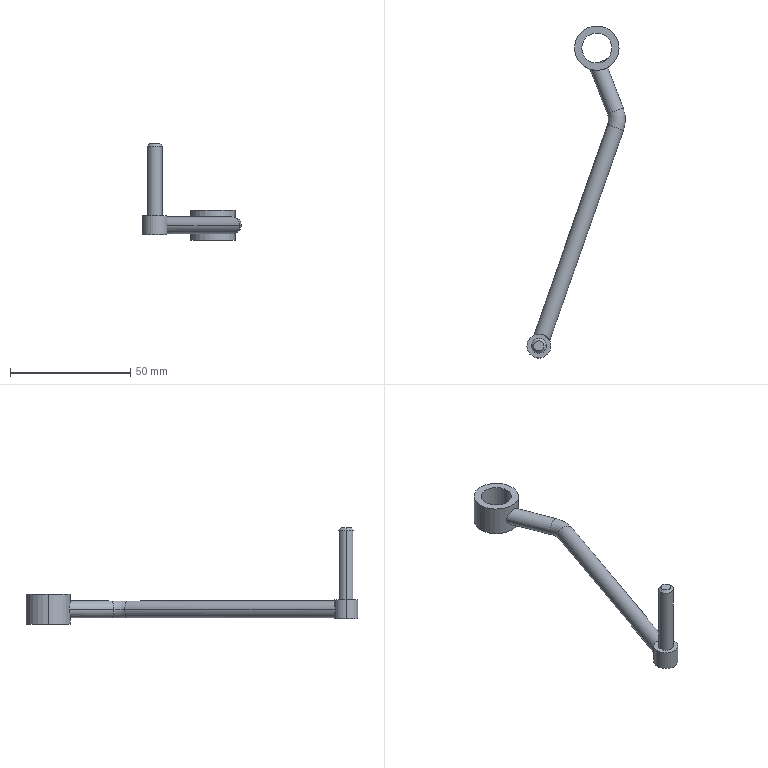Part | SolidWorks | features 3DProfileFeature 2, ICE 2, Chamfer 1, Extrusion 1, Sweep 1 | 1 solid | 24 faces | box 40.944 x 138.187 x 40.25 mm | volume 7860 mm3 | cylinder 14 | plane 6 | torus 2 | cone 2 | commonest cylinder face diameters 7 x6 6.192 x2 10 x2 12.5 x2 18.5 x2
STEP:
#1=CARTESIAN_POINT('',(4.41,-27.398,6.25));
#2=VERTEX_POINT('',#1);
#3=CARTESIAN_POINT('',(10.941,-24.878,6.25));
#4=VERTEX_POINT('',#3);
#5=CARTESIAN_POINT('',(7.675,-26.138,6.25));
#6=DIRECTION('',(0.3601,-0.9329,0.));
#7=DIRECTION('',(0.9329,0.3601,0.));
#8=AXIS2_PLACEMENT_3D('',#5,#6,#7);
#9=CIRCLE('',#8,3.5);
#10=EDGE_CURVE('',#2,#4,#9,.T.);
#11=ORIENTED_EDGE('',*,*,#10,.T.);
#12=CARTESIAN_POINT('',(11.085,-34.207,6.25));
#13=VERTEX_POINT('',#12);
#14=CARTESIAN_POINT('',(-1.654,-29.738,6.25));
#15=DIRECTION('',(0.,0.,-1.));
#16=DIRECTION('',(0.,1.,0.));
#17=AXIS2_PLACEMENT_3D('',#14,#15,#16);
#18=CIRCLE('',#17,13.5);
#19=EDGE_CURVE('',#4,#13,#18,.T.);
#20=ORIENTED_EDGE('',*,*,#19,.T.);
#21=CARTESIAN_POINT('',(4.48,-31.89,6.25));
#22=VERTEX_POINT('',#21);
#23=CARTESIAN_POINT('',(7.782,-33.048,6.25));
#24=DIRECTION('',(-0.331,-0.9436,0.));
#25=DIRECTION('',(0.9436,-0.331,0.));
#26=AXIS2_PLACEMENT_3D('',#23,#24,#25);
#27=CIRCLE('',#26,3.5);
#28=EDGE_CURVE('',#22,#13,#27,.T.);
#29=ORIENTED_EDGE('',*,*,#28,.F.);
#30=CARTESIAN_POINT('',(-1.654,-29.738,6.25));
#31=DIRECTION('',(0.,0.,-1.));
#32=DIRECTION('',(0.,1.,0.));
#33=AXIS2_PLACEMENT_3D('',#30,#31,#32);
#34=CIRCLE('',#33,6.5);
#35=EDGE_CURVE('',#2,#22,#34,.T.);
#36=ORIENTED_EDGE('',*,*,#35,.F.);
#37=EDGE_LOOP('',(#11,#20,#29,#36));
#38=FACE_OUTER_BOUND('',#37,.T.);
#39=CARTESIAN_POINT('',(-1.654,-29.738,6.25));
#40=DIRECTION('',(0.,0.,-1.));
#41=DIRECTION('',(0.,1.,0.));
#42=AXIS2_PLACEMENT_3D('',#39,#40,#41);
#43=TOROIDAL_SURFACE('',#42,10.,3.5);
#44=ADVANCED_FACE('',(#38),#43,.T.);
#45=CARTESIAN_POINT('',(-22.001,-123.937,40.25));
#46=VERTEX_POINT('',#45);
#47=CARTESIAN_POINT('',(-26.194,-123.937,40.25));
#48=VERTEX_POINT('',#47);
#49=CARTESIAN_POINT('',(-24.097,-123.937,40.25));
#50=DIRECTION('',(0.,0.,1.));
#51=DIRECTION('',(1.,0.,0.));
#52=AXIS2_PLACEMENT_3D('',#49,#50,#51);
#53=CIRCLE('',#52,2.096);
#54=EDGE_CURVE('',#46,#48,#53,.T.);
#55=ORIENTED_EDGE('',*,*,#54,.F.);
#56=CARTESIAN_POINT('',(-21.001,-123.937,39.25));
#57=VERTEX_POINT('',#56);
#58=CARTESIAN_POINT('',(-22.001,-123.937,40.25));
#59=DIRECTION('',(0.7071,0.,-0.7071));
#60=VECTOR('',#59,1000.);
#61=LINE('',#58,#60);
#62=EDGE_CURVE('',#46,#57,#61,.T.);
#63=ORIENTED_EDGE('',*,*,#62,.T.);
#64=CARTESIAN_POINT('',(-27.194,-123.937,39.25));
#65=VERTEX_POINT('',#64);
#66=CARTESIAN_POINT('',(-24.097,-123.937,39.25));
#67=DIRECTION('',(0.,0.,-1.));
#68=DIRECTION('',(1.,0.,0.));
#69=AXIS2_PLACEMENT_3D('',#66,#67,#68);
#70=CIRCLE('',#69,3.096);
#71=EDGE_CURVE('',#65,#57,#70,.T.);
#72=ORIENTED_EDGE('',*,*,#71,.F.);
#73=CARTESIAN_POINT('',(-26.194,-123.937,40.25));
#74=DIRECTION('',(-0.7071,0.,-0.7071));
#75=VECTOR('',#74,1000.);
#76=LINE('',#73,#75);
#77=EDGE_CURVE('',#48,#65,#76,.T.);
#78=ORIENTED_EDGE('',*,*,#77,.F.);
#79=EDGE_LOOP('',(#55,#63,#72,#78));
#80=FACE_OUTER_BOUND('',#79,.T.);
#81=CARTESIAN_POINT('',(-24.097,-123.937,40.25));
#82=DIRECTION('',(0.,0.,-1.));
#83=DIRECTION('',(-1.,0.,0.));
#84=AXIS2_PLACEMENT_3D('',#81,#82,#83);
#85=CONICAL_SURFACE('',#84,2.096,0.7854);
#86=ADVANCED_FACE('',(#80),#85,.T.);
#87=ORIENTED_EDGE('',*,*,#71,.T.);
#88=CARTESIAN_POINT('',(-21.001,-123.937,10.25));
#89=VERTEX_POINT('',#88);
#90=CARTESIAN_POINT('',(-21.001,-123.937,40.25));
#91=DIRECTION('',(0.,0.,-1.));
#92=VECTOR('',#91,1000.);
#93=LINE('',#90,#92);
#94=EDGE_CURVE('',#57,#89,#93,.T.);
#95=ORIENTED_EDGE('',*,*,#94,.T.);
#96=CARTESIAN_POINT('',(-27.194,-123.937,10.25));
#97=VERTEX_POINT('',#96);
#98=CARTESIAN_POINT('',(-24.097,-123.937,10.25));
#99=DIRECTION('',(0.,0.,1.));
#100=DIRECTION('',(1.,0.,0.));
#101=AXIS2_PLACEMENT_3D('',#98,#99,#100);
#102=CIRCLE('',#101,3.096);
#103=EDGE_CURVE('',#89,#97,#102,.T.);
#104=ORIENTED_EDGE('',*,*,#103,.T.);
#105=CARTESIAN_POINT('',(-27.194,-123.937,40.25));
#106=DIRECTION('',(0.,0.,-1.));
#107=VECTOR('',#106,1000.);
#108=LINE('',#105,#107);
#109=EDGE_CURVE('',#65,#97,#108,.T.);
#110=ORIENTED_EDGE('',*,*,#109,.F.);
#111=EDGE_LOOP('',(#87,#95,#104,#110));
#112=FACE_OUTER_BOUND('',#111,.T.);
#113=CARTESIAN_POINT('',(-24.097,-123.937,40.25));
#114=DIRECTION('',(0.,0.,-1.));
#115=DIRECTION('',(-1.,0.,0.));
#116=AXIS2_PLACEMENT_3D('',#113,#114,#115);
#117=CYLINDRICAL_SURFACE('',#116,3.096);
#118=ADVANCED_FACE('',(#112),#117,.T.);
#119=CARTESIAN_POINT('',(-19.613,-121.726,6.25));
#120=VERTEX_POINT('',#119);
#121=CARTESIAN_POINT('',(-26.218,-119.409,6.25));
#122=VERTEX_POINT('',#121);
#123=CARTESIAN_POINT('',(-19.613,-121.726,6.25));
#124=CARTESIAN_POINT('',(-19.613,-121.726,6.009));
#125=CARTESIAN_POINT('',(-19.628,-121.695,5.775));
#126=CARTESIAN_POINT('',(-19.687,-121.58,5.318));
#127=CARTESIAN_POINT('',(-19.732,-121.496,5.095));
#128=CARTESIAN_POINT('',(-19.849,-121.298,4.679));
#129=CARTESIAN_POINT('',(-19.922,-121.182,4.481));
#130=CARTESIAN_POINT('',(-20.097,-120.933,4.113));
#131=CARTESIAN_POINT('',(-20.199,-120.801,3.943));
#132=CARTESIAN_POINT('',(-20.433,-120.53,3.629));
#133=CARTESIAN_POINT('',(-20.567,-120.39,3.485));
#134=CARTESIAN_POINT('',(-20.862,-120.119,3.234));
#135=CARTESIAN_POINT('',(-21.024,-119.987,3.125));
#136=CARTESIAN_POINT('',(-21.382,-119.732,2.943));
#137=CARTESIAN_POINT('',(-21.58,-119.611,2.871));
#138=CARTESIAN_POINT('',(-21.992,-119.396,2.776));
#139=CARTESIAN_POINT('',(-22.213,-119.299,2.75));
#140=CARTESIAN_POINT('',(-22.664,-119.141,2.75));
#141=CARTESIAN_POINT('',(-22.891,-119.079,2.774));
#142=CARTESIAN_POINT('',(-23.351,-118.987,2.869));
#143=CARTESIAN_POINT('',(-23.58,-118.959,2.94));
#144=CARTESIAN_POINT('',(-24.02,-118.933,3.12));
#145=CARTESIAN_POINT('',(-24.235,-118.935,3.231));
#146=CARTESIAN_POINT('',(-24.638,-118.962,3.484));
#147=CARTESIAN_POINT('',(-24.828,-118.987,3.626));
#148=CARTESIAN_POINT('',(-25.183,-119.053,3.942));
#149=CARTESIAN_POINT('',(-25.345,-119.093,4.113));
#150=CARTESIAN_POINT('',(-25.635,-119.177,4.479));
#151=CARTESIAN_POINT('',(-25.765,-119.222,4.676));
#152=CARTESIAN_POINT('',(-25.982,-119.304,5.095));
#153=CARTESIAN_POINT('',(-26.068,-119.341,5.314));
#154=CARTESIAN_POINT('',(-26.157,-119.381,5.659));
#155=CARTESIAN_POINT('',(-26.18,-119.391,5.777));
#156=CARTESIAN_POINT('',(-26.211,-119.405,6.013));
#157=CARTESIAN_POINT('',(-26.218,-119.409,6.132));
#158=CARTESIAN_POINT('',(-26.218,-119.409,6.25));
#159=B_SPLINE_CURVE_WITH_KNOTS('',3,(#123,#124,#125,#126,#127,#128,#129,#130,#131,#132,#133,#134,#135,#136,#137,#138,#139,#140,#141,#142,#143,#144,#145,#146,#147,#148,#149,#150,#151,#152,#153,#154,#155,#156,#157,#158),.UNSPECIFIED.,.F.,.F.,(4,2,2,2,2,2,2,2,2,2,2,2,2,2,2,2,2,4),(0.,0.0007095,0.001419,0.002128,0.002838,0.003547,0.004257,0.004966,0.005676,0.006385,0.007095,0.007804,0.008514,0.009223,0.009933,0.01064,0.011,0.01135),.UNSPECIFIED.);
#160=EDGE_CURVE('',#120,#122,#159,.T.);
#161=ORIENTED_EDGE('',*,*,#160,.F.);
#162=CARTESIAN_POINT('',(-26.218,-119.409,6.25));
#163=CARTESIAN_POINT('',(-26.218,-119.409,6.486));
#164=CARTESIAN_POINT('',(-26.187,-119.394,6.727));
#165=CARTESIAN_POINT('',(-26.068,-119.341,7.186));
#166=CARTESIAN_POINT('',(-25.981,-119.304,7.407));
#167=CARTESIAN_POINT('',(-25.764,-119.221,7.826));
#168=CARTESIAN_POINT('',(-25.636,-119.177,8.02));
#169=CARTESIAN_POINT('',(-25.346,-119.093,8.386));
#170=CARTESIAN_POINT('',(-25.182,-119.053,8.559));
#171=CARTESIAN_POINT('',(-24.83,-118.987,8.872));
#172=CARTESIAN_POINT('',(-24.641,-118.962,9.013));
#173=CARTESIAN_POINT('',(-24.239,-118.935,9.266));
#174=CARTESIAN_POINT('',(-24.024,-118.933,9.378));
#175=CARTESIAN_POINT('',(-23.586,-118.958,9.558));
#176=CARTESIAN_POINT('',(-23.359,-118.986,9.629));
#177=CARTESIAN_POINT('',(-22.898,-119.077,9.726));
#178=CARTESIAN_POINT('',(-22.671,-119.139,9.75));
#179=CARTESIAN_POINT('',(-22.222,-119.296,9.75));
#180=CARTESIAN_POINT('',(-22.,-119.392,9.726));
#181=CARTESIAN_POINT('',(-21.587,-119.607,9.631));
#182=CARTESIAN_POINT('',(-21.39,-119.727,9.56));
#183=CARTESIAN_POINT('',(-21.029,-119.983,9.378));
#184=CARTESIAN_POINT('',(-20.866,-120.116,9.269));
#185=CARTESIAN_POINT('',(-20.567,-120.391,9.015));
#186=CARTESIAN_POINT('',(-20.433,-120.53,8.871));
#187=CARTESIAN_POINT('',(-20.199,-120.8,8.558));
#188=CARTESIAN_POINT('',(-20.097,-120.934,8.386));
#189=CARTESIAN_POINT('',(-19.922,-121.183,8.018));
#190=CARTESIAN_POINT('',(-19.85,-121.297,7.823));
#191=CARTESIAN_POINT('',(-19.762,-121.445,7.513));
#192=CARTESIAN_POINT('',(-19.737,-121.491,7.407));
#193=CARTESIAN_POINT('',(-19.692,-121.572,7.186));
#194=CARTESIAN_POINT('',(-19.673,-121.608,7.072));
#195=CARTESIAN_POINT('',(-19.628,-121.694,6.727));
#196=CARTESIAN_POINT('',(-19.613,-121.726,6.491));
#197=CARTESIAN_POINT('',(-19.613,-121.726,6.25));
#198=B_SPLINE_CURVE_WITH_KNOTS('',3,(#162,#163,#164,#165,#166,#167,#168,#169,#170,#171,#172,#173,#174,#175,#176,#177,#178,#179,#180,#181,#182,#183,#184,#185,#186,#187,#188,#189,#190,#191,#192,#193,#194,#195,#196,#197),.UNSPECIFIED.,.F.,.F.,(4,2,2,2,2,2,2,2,2,2,2,2,2,2,2,2,2,4),(0.01135,0.01206,0.01277,0.01348,0.01419,0.01489,0.0156,0.01631,0.01702,0.01773,0.01844,0.01914,0.01985,0.02056,0.02127,0.02162,0.02198,0.02269),.UNSPECIFIED.);
#199=EDGE_CURVE('',#122,#120,#198,.T.);
#200=ORIENTED_EDGE('',*,*,#199,.F.);
#201=EDGE_LOOP('',(#161,#200));
#202=FACE_BOUND('',#201,.T.);
#203=CARTESIAN_POINT('',(-19.097,-123.937,10.25));
#204=VERTEX_POINT('',#203);
#205=CARTESIAN_POINT('',(-29.097,-123.937,10.25));
#206=VERTEX_POINT('',#205);
#207=CARTESIAN_POINT('',(-24.097,-123.937,10.25));
#208=DIRECTION('',(0.,0.,1.));
#209=DIRECTION('',(1.,0.,0.));
#210=AXIS2_PLACEMENT_3D('',#207,#208,#209);
#211=CIRCLE('',#210,5.);
#212=EDGE_CURVE('',#204,#206,#211,.T.);
#213=ORIENTED_EDGE('',*,*,#212,.F.);
#214=CARTESIAN_POINT('',(-19.097,-123.937,2.25));
#215=VERTEX_POINT('',#214);
#216=CARTESIAN_POINT('',(-19.097,-123.937,10.25));
#217=DIRECTION('',(0.,0.,-1.));
#218=VECTOR('',#217,1000.);
#219=LINE('',#216,#218);
#220=EDGE_CURVE('',#204,#215,#219,.T.);
#221=ORIENTED_EDGE('',*,*,#220,.T.);
#222=CARTESIAN_POINT('',(-29.097,-123.937,2.25));
#223=VERTEX_POINT('',#222);
#224=CARTESIAN_POINT('',(-24.097,-123.937,2.25));
#225=DIRECTION('',(0.,0.,1.));
#226=DIRECTION('',(1.,0.,0.));
#227=AXIS2_PLACEMENT_3D('',#224,#225,#226);
#228=CIRCLE('',#227,5.);
#229=EDGE_CURVE('',#215,#223,#228,.T.);
#230=ORIENTED_EDGE('',*,*,#229,.T.);
#231=CARTESIAN_POINT('',(-29.097,-123.937,10.25));
#232=DIRECTION('',(0.,0.,-1.));
#233=VECTOR('',#232,1000.);
#234=LINE('',#231,#233);
#235=EDGE_CURVE('',#206,#223,#234,.T.);
#236=ORIENTED_EDGE('',*,*,#235,.F.);
#237=EDGE_LOOP('',(#213,#221,#230,#236));
#238=FACE_OUTER_BOUND('',#237,.T.);
#239=CARTESIAN_POINT('',(-24.097,-123.937,10.25));
#240=DIRECTION('',(0.,0.,-1.));
#241=DIRECTION('',(-1.,0.,0.));
#242=AXIS2_PLACEMENT_3D('',#239,#240,#241);
#243=CYLINDRICAL_SURFACE('',#242,5.);
#244=ADVANCED_FACE('',(#202,#238),#243,.T.);
#245=CARTESIAN_POINT('',(-2.756,-8.83,6.25));
#246=VERTEX_POINT('',#245);
#247=CARTESIAN_POINT('',(4.466,-8.101,6.25));
#248=VERTEX_POINT('',#247);
#249=CARTESIAN_POINT('',(-2.756,-8.83,6.25));
#250=CARTESIAN_POINT('',(-2.756,-8.83,6.484));
#251=CARTESIAN_POINT('',(-2.726,-8.839,6.723));
#252=CARTESIAN_POINT('',(-2.613,-8.873,7.179));
#253=CARTESIAN_POINT('',(-2.53,-8.898,7.4));
#254=CARTESIAN_POINT('',(-2.318,-8.956,7.819));
#255=CARTESIAN_POINT('',(-2.191,-8.988,8.015));
#256=CARTESIAN_POINT('',(-1.902,-9.054,8.383));
#257=CARTESIAN_POINT('',(-1.739,-9.087,8.554));
#258=CARTESIAN_POINT('',(-1.215,-9.177,9.017));
#259=CARTESIAN_POINT('',(-0.8076,-9.225,9.268));
#260=CARTESIAN_POINT('',(-0.1584,-9.251,9.535));
#261=CARTESIAN_POINT('',(0.06706,-9.253,9.606));
#262=CARTESIAN_POINT('',(0.5295,-9.238,9.709));
#263=CARTESIAN_POINT('',(0.7612,-9.222,9.739));
#264=CARTESIAN_POINT('',(1.226,-9.171,9.756));
#265=CARTESIAN_POINT('',(1.461,-9.137,9.743));
#266=CARTESIAN_POINT('',(1.92,-9.052,9.669));
#267=CARTESIAN_POINT('',(2.141,-9.001,9.61));
#268=CARTESIAN_POINT('',(2.567,-8.889,9.446));
#269=CARTESIAN_POINT('',(2.773,-8.827,9.34));
#270=CARTESIAN_POINT('',(3.151,-8.699,9.091));
#271=CARTESIAN_POINT('',(3.325,-8.634,8.947));
#272=CARTESIAN_POINT('',(3.643,-8.504,8.619));
#273=CARTESIAN_POINT('',(3.784,-8.442,8.439));
#274=CARTESIAN_POINT('',(4.027,-8.328,8.054));
#275=CARTESIAN_POINT('',(4.131,-8.277,7.845));
#276=CARTESIAN_POINT('',(4.297,-8.192,7.411));
#277=CARTESIAN_POINT('',(4.36,-8.158,7.188));
#278=CARTESIAN_POINT('',(4.444,-8.113,6.726));
#279=CARTESIAN_POINT('',(4.466,-8.101,6.488));
#280=CARTESIAN_POINT('',(4.466,-8.101,6.25));
#281=B_SPLINE_CURVE_WITH_KNOTS('',3,(#249,#250,#251,#252,#253,#254,#255,#256,#257,#258,#259,#260,#261,#262,#263,#264,#265,#266,#267,#268,#269,#270,#271,#272,#273,#274,#275,#276,#277,#278,#279,#280),.UNSPECIFIED.,.F.,.F.,(4,2,2,2,2,2,2,2,2,2,2,2,2,2,2,4),(0.01126,0.01196,0.01266,0.01337,0.01407,0.01547,0.01618,0.01688,0.01758,0.01828,0.01899,0.01969,0.02039,0.02109,0.0218,0.0225),.UNSPECIFIED.);
#282=EDGE_CURVE('',#246,#248,#281,.T.);
#283=ORIENTED_EDGE('',*,*,#282,.F.);
#284=CARTESIAN_POINT('',(-3.265,-7.51,6.25));
#285=DIRECTION('',(0.3601,-0.9329,0.));
#286=VECTOR('',#285,1000.);
#287=LINE('',#284,#286);
#288=EDGE_CURVE('',#246,#2,#287,.T.);
#289=ORIENTED_EDGE('',*,*,#288,.T.);
#290=CARTESIAN_POINT('',(7.675,-26.138,6.25));
#291=DIRECTION('',(0.3601,-0.9329,0.));
#292=DIRECTION('',(0.9329,0.3601,0.));
#293=AXIS2_PLACEMENT_3D('',#290,#291,#292);
#294=CIRCLE('',#293,3.5);
#295=EDGE_CURVE('',#4,#2,#294,.T.);
#296=ORIENTED_EDGE('',*,*,#295,.F.);
#297=CARTESIAN_POINT('',(3.265,-4.99,6.25));
#298=DIRECTION('',(0.3601,-0.9329,0.));
#299=VECTOR('',#298,1000.);
#300=LINE('',#297,#299);
#301=EDGE_CURVE('',#248,#4,#300,.T.);
#302=ORIENTED_EDGE('',*,*,#301,.F.);
#303=EDGE_LOOP('',(#283,#289,#296,#302));
#304=FACE_OUTER_BOUND('',#303,.T.);
#305=CARTESIAN_POINT('',(0.,-6.25,6.25));
#306=DIRECTION('',(0.3601,-0.9329,0.));
#307=DIRECTION('',(0.9329,0.3601,0.));
#308=AXIS2_PLACEMENT_3D('',#305,#306,#307);
#309=CYLINDRICAL_SURFACE('',#308,3.5);
#310=ADVANCED_FACE('',(#304),#309,.T.);
#311=CARTESIAN_POINT('',(0.,-6.25,2.75));
#312=VERTEX_POINT('',#311);
#313=CARTESIAN_POINT('',(3.265,-4.99,6.25));
#314=VERTEX_POINT('',#313);
#315=CARTESIAN_POINT('',(0.,-6.25,6.25));
#316=DIRECTION('',(0.3601,-0.9329,0.));
#317=DIRECTION('',(0.9329,0.3601,0.));
#318=AXIS2_PLACEMENT_3D('',#315,#316,#317);
#319=CIRCLE('',#318,3.5);
#320=EDGE_CURVE('',#312,#314,#319,.T.);
#321=ORIENTED_EDGE('',*,*,#320,.T.);
#322=CARTESIAN_POINT('',(3.371,-5.263,6.25));
#323=VERTEX_POINT('',#322);
#324=CARTESIAN_POINT('',(3.265,-4.99,6.25));
#325=DIRECTION('',(0.3601,-0.9329,0.));
#326=VECTOR('',#325,1000.);
#327=LINE('',#324,#326);
#328=EDGE_CURVE('',#314,#323,#327,.T.);
#329=ORIENTED_EDGE('',*,*,#328,.T.);
#330=CARTESIAN_POINT('',(3.371,-5.263,6.25));
#331=CARTESIAN_POINT('',(3.371,-5.263,6.017));
#332=CARTESIAN_POINT('',(3.351,-5.276,5.787));
#333=CARTESIAN_POINT('',(3.273,-5.325,5.336));
#334=CARTESIAN_POINT('',(3.213,-5.361,5.112));
#335=CARTESIAN_POINT('',(3.057,-5.452,4.686));
#336=CARTESIAN_POINT('',(2.961,-5.506,4.484));
#337=CARTESIAN_POINT('',(2.73,-5.624,4.101));
#338=CARTESIAN_POINT('',(2.594,-5.689,3.92));
#339=CARTESIAN_POINT('',(2.293,-5.817,3.597));
#340=CARTESIAN_POINT('',(2.125,-5.881,3.452));
#341=CARTESIAN_POINT('',(1.755,-6.002,3.196));
#342=CARTESIAN_POINT('',(1.557,-6.057,3.09));
#343=CARTESIAN_POINT('',(1.14,-6.149,2.919));
#344=CARTESIAN_POINT('',(0.9171,-6.187,2.855));
#345=CARTESIAN_POINT('',(0.4638,-6.237,2.77));
#346=CARTESIAN_POINT('',(0.2336,-6.25,2.75));
#347=CARTESIAN_POINT('',(0.,-6.25,2.75));
#348=B_SPLINE_CURVE_WITH_KNOTS('',3,(#330,#331,#332,#333,#334,#335,#336,#337,#338,#339,#340,#341,#342,#343,#344,#345,#346,#347),.UNSPECIFIED.,.F.,.F.,(4,2,2,2,2,2,2,2,4),(0.005526,0.006217,0.006908,0.007599,0.00829,0.008981,0.009672,0.01036,0.01105),.UNSPECIFIED.);
#349=EDGE_CURVE('',#323,#312,#348,.T.);
#350=ORIENTED_EDGE('',*,*,#349,.T.);
#351=EDGE_LOOP('',(#321,#329,#350));
#352=FACE_OUTER_BOUND('',#351,.T.);
#353=CARTESIAN_POINT('',(0.,-6.25,6.25));
#354=DIRECTION('',(0.3601,-0.9329,0.));
#355=DIRECTION('',(0.9329,0.3601,0.));
#356=AXIS2_PLACEMENT_3D('',#353,#354,#355);
#357=CYLINDRICAL_SURFACE('',#356,3.5);
#358=ADVANCED_FACE('',(#352),#357,.T.);
#359=CARTESIAN_POINT('',(9.25,0.,12.5));
#360=VERTEX_POINT('',#359);
#361=CARTESIAN_POINT('',(-9.25,0.,12.5));
#362=VERTEX_POINT('',#361);
#363=CARTESIAN_POINT('',(0.,0.,12.5));
#364=DIRECTION('',(0.,0.,1.));
#365=DIRECTION('',(1.,0.,0.));
#366=AXIS2_PLACEMENT_3D('',#363,#364,#365);
#367=CIRCLE('',#366,9.25);
#368=EDGE_CURVE('',#360,#362,#367,.T.);
#369=ORIENTED_EDGE('',*,*,#368,.F.);
#370=CARTESIAN_POINT('',(9.25,0.,0.));
#371=VERTEX_POINT('',#370);
#372=CARTESIAN_POINT('',(9.25,0.,12.5));
#373=DIRECTION('',(0.,0.,-1.));
#374=VECTOR('',#373,1000.);
#375=LINE('',#372,#374);
#376=EDGE_CURVE('',#360,#371,#375,.T.);
#377=ORIENTED_EDGE('',*,*,#376,.T.);
#378=CARTESIAN_POINT('',(-9.25,0.,0.));
#379=VERTEX_POINT('',#378);
#380=CARTESIAN_POINT('',(0.,0.,0.));
#381=DIRECTION('',(0.,0.,1.));
#382=DIRECTION('',(1.,0.,0.));
#383=AXIS2_PLACEMENT_3D('',#380,#381,#382);
#384=CIRCLE('',#383,9.25);
#385=EDGE_CURVE('',#371,#379,#384,.T.);
#386=ORIENTED_EDGE('',*,*,#385,.T.);
#387=CARTESIAN_POINT('',(-9.25,0.,12.5));
#388=DIRECTION('',(0.,0.,-1.));
#389=VECTOR('',#388,1000.);
#390=LINE('',#387,#389);
#391=EDGE_CURVE('',#362,#379,#390,.T.);
#392=ORIENTED_EDGE('',*,*,#391,.F.);
#393=EDGE_LOOP('',(#369,#377,#386,#392));
#394=FACE_OUTER_BOUND('',#393,.T.);
#395=CARTESIAN_POINT('',(0.,0.,12.5));
#396=DIRECTION('',(0.,0.,-1.));
#397=DIRECTION('',(-1.,0.,0.));
#398=AXIS2_PLACEMENT_3D('',#395,#396,#397);
#399=CYLINDRICAL_SURFACE('',#398,9.25);
#400=ADVANCED_FACE('',(#394),#399,.T.);
#401=CARTESIAN_POINT('',(0.,-6.25,9.75));
#402=VERTEX_POINT('',#401);
#403=CARTESIAN_POINT('',(0.,-6.25,9.75));
#404=CARTESIAN_POINT('',(0.2334,-6.25,9.75));
#405=CARTESIAN_POINT('',(0.4629,-6.237,9.73));
#406=CARTESIAN_POINT('',(0.9135,-6.187,9.646));
#407=CARTESIAN_POINT('',(1.137,-6.149,9.581));
#408=CARTESIAN_POINT('',(1.556,-6.057,9.411));
#409=CARTESIAN_POINT('',(1.753,-6.002,9.305));
#410=CARTESIAN_POINT('',(2.123,-5.882,9.05));
#411=CARTESIAN_POINT('',(2.292,-5.817,8.903));
#412=CARTESIAN_POINT('',(2.594,-5.689,8.58));
#413=CARTESIAN_POINT('',(2.73,-5.624,8.399));
#414=CARTESIAN_POINT('',(2.961,-5.506,8.016));
#415=CARTESIAN_POINT('',(3.057,-5.452,7.814));
#416=CARTESIAN_POINT('',(3.214,-5.361,7.387));
#417=CARTESIAN_POINT('',(3.273,-5.325,7.164));
#418=CARTESIAN_POINT('',(3.351,-5.276,6.713));
#419=CARTESIAN_POINT('',(3.371,-5.263,6.483));
#420=CARTESIAN_POINT('',(3.371,-5.263,6.25));
#421=B_SPLINE_CURVE_WITH_KNOTS('',3,(#403,#404,#405,#406,#407,#408,#409,#410,#411,#412,#413,#414,#415,#416,#417,#418,#419,#420),.UNSPECIFIED.,.F.,.F.,(4,2,2,2,2,2,2,2,4),(0.,0.0006908,0.001382,0.002072,0.002763,0.003454,0.004145,0.004835,0.005526),.UNSPECIFIED.);
#422=EDGE_CURVE('',#402,#323,#421,.T.);
#423=ORIENTED_EDGE('',*,*,#422,.F.);
#424=CARTESIAN_POINT('',(0.,-6.25,12.5));
#425=DIRECTION('',(0.,0.,-1.));
#426=VECTOR('',#425,1000.);
#427=LINE('',#424,#426);
#428=EDGE_CURVE('',#402,#312,#427,.T.);
#429=ORIENTED_EDGE('',*,*,#428,.T.);
#430=ORIENTED_EDGE('',*,*,#349,.F.);
#431=EDGE_LOOP('',(#423,#429,#430));
#432=FACE_BOUND('',#431,.T.);
#433=CARTESIAN_POINT('',(-6.25,0.,12.5));
#434=VERTEX_POINT('',#433);
#435=CARTESIAN_POINT('',(6.25,0.,12.5));
#436=VERTEX_POINT('',#435);
#437=CARTESIAN_POINT('',(0.,0.,12.5));
#438=DIRECTION('',(0.,0.,1.));
#439=DIRECTION('',(1.,0.,0.));
#440=AXIS2_PLACEMENT_3D('',#437,#438,#439);
#441=CIRCLE('',#440,6.25);
#442=EDGE_CURVE('',#434,#436,#441,.T.);
#443=ORIENTED_EDGE('',*,*,#442,.T.);
#444=CARTESIAN_POINT('',(6.25,0.,0.));
#445=VERTEX_POINT('',#444);
#446=CARTESIAN_POINT('',(6.25,0.,12.5));
#447=DIRECTION('',(0.,0.,-1.));
#448=VECTOR('',#447,1000.);
#449=LINE('',#446,#448);
#450=EDGE_CURVE('',#436,#445,#449,.T.);
#451=ORIENTED_EDGE('',*,*,#450,.T.);
#452=CARTESIAN_POINT('',(-6.25,0.,0.));
#453=VERTEX_POINT('',#452);
#454=CARTESIAN_POINT('',(0.,0.,0.));
#455=DIRECTION('',(0.,0.,1.));
#456=DIRECTION('',(1.,0.,0.));
#457=AXIS2_PLACEMENT_3D('',#454,#455,#456);
#458=CIRCLE('',#457,6.25);
#459=EDGE_CURVE('',#453,#445,#458,.T.);
#460=ORIENTED_EDGE('',*,*,#459,.F.);
#461=CARTESIAN_POINT('',(-6.25,0.,12.5));
#462=DIRECTION('',(0.,0.,-1.));
#463=VECTOR('',#462,1000.);
#464=LINE('',#461,#463);
#465=EDGE_CURVE('',#434,#453,#464,.T.);
#466=ORIENTED_EDGE('',*,*,#465,.F.);
#467=EDGE_LOOP('',(#443,#451,#460,#466));
#468=FACE_OUTER_BOUND('',#467,.T.);
#469=CARTESIAN_POINT('',(0.,0.,12.5));
#470=DIRECTION('',(0.,0.,-1.));
#471=DIRECTION('',(-1.,0.,0.));
#472=AXIS2_PLACEMENT_3D('',#469,#470,#471);
#473=CYLINDRICAL_SURFACE('',#472,6.25);
#474=ADVANCED_FACE('',(#432,#468),#473,.F.);
#475=CARTESIAN_POINT('',(7.782,-33.048,6.25));
#476=DIRECTION('',(-0.331,-0.9436,0.));
#477=DIRECTION('',(0.9436,-0.331,0.));
#478=AXIS2_PLACEMENT_3D('',#475,#476,#477);
#479=CIRCLE('',#478,3.5);
#480=EDGE_CURVE('',#13,#22,#479,.T.);
#481=ORIENTED_EDGE('',*,*,#480,.T.);
#482=CARTESIAN_POINT('',(4.48,-31.89,6.25));
#483=DIRECTION('',(-0.331,-0.9436,0.));
#484=VECTOR('',#483,1000.);
#485=LINE('',#482,#484);
#486=EDGE_CURVE('',#22,#122,#485,.T.);
#487=ORIENTED_EDGE('',*,*,#486,.T.);
#488=ORIENTED_EDGE('',*,*,#199,.T.);
#489=CARTESIAN_POINT('',(11.085,-34.207,6.25));
#490=DIRECTION('',(-0.331,-0.9436,0.));
#491=VECTOR('',#490,1000.);
#492=LINE('',#489,#491);
#493=EDGE_CURVE('',#13,#120,#492,.T.);
#494=ORIENTED_EDGE('',*,*,#493,.F.);
#495=EDGE_LOOP('',(#481,#487,#488,#494));
#496=FACE_OUTER_BOUND('',#495,.T.);
#497=CARTESIAN_POINT('',(7.782,-33.048,6.25));
#498=DIRECTION('',(-0.331,-0.9436,0.));
#499=DIRECTION('',(0.9436,-0.331,0.));
#500=AXIS2_PLACEMENT_3D('',#497,#498,#499);
#501=CYLINDRICAL_SURFACE('',#500,3.5);
#502=ADVANCED_FACE('',(#496),#501,.T.);
#503=ORIENTED_EDGE('',*,*,#486,.F.);
#504=ORIENTED_EDGE('',*,*,#28,.T.);
#505=ORIENTED_EDGE('',*,*,#493,.T.);
#506=ORIENTED_EDGE('',*,*,#160,.T.);
#507=EDGE_LOOP('',(#503,#504,#505,#506));
#508=FACE_OUTER_BOUND('',#507,.T.);
#509=CARTESIAN_POINT('',(7.782,-33.048,6.25));
#510=DIRECTION('',(-0.331,-0.9436,0.));
#511=DIRECTION('',(0.9436,-0.331,0.));
#512=AXIS2_PLACEMENT_3D('',#509,#510,#511);
#513=CYLINDRICAL_SURFACE('',#512,3.5);
#514=ADVANCED_FACE('',(#508),#513,.T.);
#515=ORIENTED_EDGE('',*,*,#450,.F.);
#516=CARTESIAN_POINT('',(0.,0.,12.5));
#517=DIRECTION('',(0.,0.,1.));
#518=DIRECTION('',(1.,0.,0.));
#519=AXIS2_PLACEMENT_3D('',#516,#517,#518);
#520=CIRCLE('',#519,6.25);
#521=EDGE_CURVE('',#436,#434,#520,.T.);
#522=ORIENTED_EDGE('',*,*,#521,.T.);
#523=ORIENTED_EDGE('',*,*,#465,.T.);
#524=CARTESIAN_POINT('',(0.,0.,0.));
#525=DIRECTION('',(0.,0.,1.));
#526=DIRECTION('',(1.,0.,0.));
#527=AXIS2_PLACEMENT_3D('',#524,#525,#526);
#528=CIRCLE('',#527,6.25);
#529=EDGE_CURVE('',#445,#453,#528,.T.);
#530=ORIENTED_EDGE('',*,*,#529,.F.);
#531=EDGE_LOOP('',(#515,#522,#523,#530));
#532=FACE_OUTER_BOUND('',#531,.T.);
#533=CARTESIAN_POINT('',(0.,0.,12.5));
#534=DIRECTION('',(0.,0.,-1.));
#535=DIRECTION('',(-1.,0.,0.));
#536=AXIS2_PLACEMENT_3D('',#533,#534,#535);
#537=CYLINDRICAL_SURFACE('',#536,6.25);
#538=ADVANCED_FACE('',(#532),#537,.F.);
#539=CARTESIAN_POINT('',(0.,0.,12.5));
#540=DIRECTION('',(0.,0.,1.));
#541=DIRECTION('',(1.,0.,0.));
#542=AXIS2_PLACEMENT_3D('',#539,#540,#541);
#543=CIRCLE('',#542,9.25);
#544=EDGE_CURVE('',#362,#360,#543,.T.);
#545=ORIENTED_EDGE('',*,*,#544,.T.);
#546=ORIENTED_EDGE('',*,*,#368,.T.);
#547=EDGE_LOOP('',(#545,#546));
#548=FACE_OUTER_BOUND('',#547,.T.);
#549=ORIENTED_EDGE('',*,*,#442,.F.);
#550=ORIENTED_EDGE('',*,*,#521,.F.);
#551=EDGE_LOOP('',(#549,#550));
#552=FACE_BOUND('',#551,.T.);
#553=CARTESIAN_POINT('',(0.,0.,12.5));
#554=DIRECTION('',(0.,0.,1.));
#555=DIRECTION('',(1.,0.,0.));
#556=AXIS2_PLACEMENT_3D('',#553,#554,#555);
#557=PLANE('',#556);
#558=ADVANCED_FACE('',(#548,#552),#557,.T.);
#559=CARTESIAN_POINT('',(0.,0.,0.));
#560=DIRECTION('',(0.,0.,1.));
#561=DIRECTION('',(1.,0.,0.));
#562=AXIS2_PLACEMENT_3D('',#559,#560,#561);
#563=CIRCLE('',#562,9.25);
#564=EDGE_CURVE('',#379,#371,#563,.T.);
#565=ORIENTED_EDGE('',*,*,#564,.F.);
#566=ORIENTED_EDGE('',*,*,#385,.F.);
#567=EDGE_LOOP('',(#565,#566));
#568=FACE_OUTER_BOUND('',#567,.T.);
#569=ORIENTED_EDGE('',*,*,#459,.T.);
#570=ORIENTED_EDGE('',*,*,#529,.T.);
#571=EDGE_LOOP('',(#569,#570));
#572=FACE_BOUND('',#571,.T.);
#573=CARTESIAN_POINT('',(0.,0.,0.));
#574=DIRECTION('',(0.,0.,1.));
#575=DIRECTION('',(1.,0.,0.));
#576=AXIS2_PLACEMENT_3D('',#573,#574,#575);
#577=PLANE('',#576);
#578=ADVANCED_FACE('',(#568,#572),#577,.F.);
#579=ORIENTED_EDGE('',*,*,#376,.F.);
#580=ORIENTED_EDGE('',*,*,#544,.F.);
#581=ORIENTED_EDGE('',*,*,#391,.T.);
#582=ORIENTED_EDGE('',*,*,#564,.T.);
#583=EDGE_LOOP('',(#579,#580,#581,#582));
#584=FACE_OUTER_BOUND('',#583,.T.);
#585=CARTESIAN_POINT('',(4.466,-8.101,6.25));
#586=CARTESIAN_POINT('',(4.466,-8.101,6.012));
#587=CARTESIAN_POINT('',(4.445,-8.112,5.778));
#588=CARTESIAN_POINT('',(4.361,-8.158,5.318));
#589=CARTESIAN_POINT('',(4.298,-8.191,5.09));
#590=CARTESIAN_POINT('',(4.132,-8.276,4.657));
#591=CARTESIAN_POINT('',(4.03,-8.327,4.452));
#592=CARTESIAN_POINT('',(3.786,-8.441,4.064));
#593=CARTESIAN_POINT('',(3.644,-8.504,3.882));
#594=CARTESIAN_POINT('',(3.33,-8.632,3.558));
#595=CARTESIAN_POINT('',(3.157,-8.697,3.413));
#596=CARTESIAN_POINT('',(2.775,-8.826,3.16));
#597=CARTESIAN_POINT('',(2.573,-8.888,3.056));
#598=CARTESIAN_POINT('',(2.148,-9.,2.892));
#599=CARTESIAN_POINT('',(1.922,-9.051,2.831));
#600=CARTESIAN_POINT('',(1.464,-9.136,2.758));
#601=CARTESIAN_POINT('',(1.232,-9.171,2.744));
#602=CARTESIAN_POINT('',(0.7621,-9.222,2.761));
#603=CARTESIAN_POINT('',(0.5262,-9.238,2.792));
#604=CARTESIAN_POINT('',(0.06749,-9.253,2.894));
#605=CARTESIAN_POINT('',(-0.159,-9.251,2.965));
#606=CARTESIAN_POINT('',(-0.5968,-9.233,3.145));
#607=CARTESIAN_POINT('',(-0.8055,-9.217,3.252));
#608=CARTESIAN_POINT('',(-1.203,-9.174,3.5));
#609=CARTESIAN_POINT('',(-1.394,-9.146,3.641));
#610=CARTESIAN_POINT('',(-1.744,-9.086,3.951));
#611=CARTESIAN_POINT('',(-1.903,-9.053,4.119));
#612=CARTESIAN_POINT('',(-2.191,-8.988,4.484));
#613=CARTESIAN_POINT('',(-2.32,-8.955,4.684));
#614=CARTESIAN_POINT('',(-2.53,-8.898,5.102));
#615=CARTESIAN_POINT('',(-2.613,-8.873,5.321));
#616=CARTESIAN_POINT('',(-2.727,-8.839,5.782));
#617=CARTESIAN_POINT('',(-2.756,-8.83,6.015));
#618=CARTESIAN_POINT('',(-2.756,-8.83,6.25));
#619=B_SPLINE_CURVE_WITH_KNOTS('',3,(#585,#586,#587,#588,#589,#590,#591,#592,#593,#594,#595,#596,#597,#598,#599,#600,#601,#602,#603,#604,#605,#606,#607,#608,#609,#610,#611,#612,#613,#614,#615,#616,#617,#618),.UNSPECIFIED.,.F.,.F.,(4,2,2,2,2,2,2,2,2,2,2,2,2,2,2,2,4),(0.,0.0007037,0.001407,0.002111,0.002815,0.003519,0.004222,0.004926,0.00563,0.006334,0.007037,0.007741,0.008445,0.009149,0.009852,0.01056,0.01126),.UNSPECIFIED.);
#620=EDGE_CURVE('',#248,#246,#619,.T.);
#621=ORIENTED_EDGE('',*,*,#620,.T.);
#622=ORIENTED_EDGE('',*,*,#282,.T.);
#623=EDGE_LOOP('',(#621,#622));
#624=FACE_BOUND('',#623,.T.);
#625=CARTESIAN_POINT('',(0.,0.,12.5));
#626=DIRECTION('',(0.,0.,-1.));
#627=DIRECTION('',(-1.,0.,0.));
#628=AXIS2_PLACEMENT_3D('',#625,#626,#627);
#629=CYLINDRICAL_SURFACE('',#628,9.25);
#630=ADVANCED_FACE('',(#584,#624),#629,.T.);
#631=ORIENTED_EDGE('',*,*,#328,.F.);
#632=CARTESIAN_POINT('',(0.,-6.25,6.25));
#633=DIRECTION('',(0.3601,-0.9329,0.));
#634=DIRECTION('',(0.9329,0.3601,0.));
#635=AXIS2_PLACEMENT_3D('',#632,#633,#634);
#636=CIRCLE('',#635,3.5);
#637=EDGE_CURVE('',#314,#402,#636,.T.);
#638=ORIENTED_EDGE('',*,*,#637,.T.);
#639=ORIENTED_EDGE('',*,*,#422,.T.);
#640=EDGE_LOOP('',(#631,#638,#639));
#641=FACE_OUTER_BOUND('',#640,.T.);
#642=CARTESIAN_POINT('',(0.,-6.25,6.25));
#643=DIRECTION('',(0.3601,-0.9329,0.));
#644=DIRECTION('',(0.9329,0.3601,0.));
#645=AXIS2_PLACEMENT_3D('',#642,#643,#644);
#646=CYLINDRICAL_SURFACE('',#645,3.5);
#647=ADVANCED_FACE('',(#641),#646,.T.);
#648=ORIENTED_EDGE('',*,*,#428,.F.);
#649=ORIENTED_EDGE('',*,*,#637,.F.);
#650=ORIENTED_EDGE('',*,*,#320,.F.);
#651=EDGE_LOOP('',(#648,#649,#650));
#652=FACE_OUTER_BOUND('',#651,.T.);
#653=CARTESIAN_POINT('',(0.,-6.25,6.25));
#654=DIRECTION('',(0.3601,-0.9329,0.));
#655=DIRECTION('',(0.9329,0.3601,0.));
#656=AXIS2_PLACEMENT_3D('',#653,#654,#655);
#657=PLANE('',#656);
#658=ADVANCED_FACE('',(#652),#657,.F.);
#659=ORIENTED_EDGE('',*,*,#288,.F.);
#660=ORIENTED_EDGE('',*,*,#620,.F.);
#661=ORIENTED_EDGE('',*,*,#301,.T.);
#662=ORIENTED_EDGE('',*,*,#10,.F.);
#663=EDGE_LOOP('',(#659,#660,#661,#662));
#664=FACE_OUTER_BOUND('',#663,.T.);
#665=CARTESIAN_POINT('',(0.,-6.25,6.25));
#666=DIRECTION('',(0.3601,-0.9329,0.));
#667=DIRECTION('',(0.9329,0.3601,0.));
#668=AXIS2_PLACEMENT_3D('',#665,#666,#667);
#669=CYLINDRICAL_SURFACE('',#668,3.5);
#670=ADVANCED_FACE('',(#664),#669,.T.);
#671=ORIENTED_EDGE('',*,*,#19,.F.);
#672=ORIENTED_EDGE('',*,*,#295,.T.);
#673=ORIENTED_EDGE('',*,*,#35,.T.);
#674=ORIENTED_EDGE('',*,*,#480,.F.);
#675=EDGE_LOOP('',(#671,#672,#673,#674));
#676=FACE_OUTER_BOUND('',#675,.T.);
#677=CARTESIAN_POINT('',(-1.654,-29.738,6.25));
#678=DIRECTION('',(0.,0.,-1.));
#679=DIRECTION('',(0.,1.,0.));
#680=AXIS2_PLACEMENT_3D('',#677,#678,#679);
#681=TOROIDAL_SURFACE('',#680,10.,3.5);
#682=ADVANCED_FACE('',(#676),#681,.T.);
#683=ORIENTED_EDGE('',*,*,#220,.F.);
#684=CARTESIAN_POINT('',(-24.097,-123.937,10.25));
#685=DIRECTION('',(0.,0.,1.));
#686=DIRECTION('',(1.,0.,0.));
#687=AXIS2_PLACEMENT_3D('',#684,#685,#686);
#688=CIRCLE('',#687,5.);
#689=EDGE_CURVE('',#206,#204,#688,.T.);
#690=ORIENTED_EDGE('',*,*,#689,.F.);
#691=ORIENTED_EDGE('',*,*,#235,.T.);
#692=CARTESIAN_POINT('',(-24.097,-123.937,2.25));
#693=DIRECTION('',(0.,0.,1.));
#694=DIRECTION('',(1.,0.,0.));
#695=AXIS2_PLACEMENT_3D('',#692,#693,#694);
#696=CIRCLE('',#695,5.);
#697=EDGE_CURVE('',#223,#215,#696,.T.);
#698=ORIENTED_EDGE('',*,*,#697,.T.);
#699=EDGE_LOOP('',(#683,#690,#691,#698));
#700=FACE_OUTER_BOUND('',#699,.T.);
#701=CARTESIAN_POINT('',(-24.097,-123.937,10.25));
#702=DIRECTION('',(0.,0.,-1.));
#703=DIRECTION('',(-1.,0.,0.));
#704=AXIS2_PLACEMENT_3D('',#701,#702,#703);
#705=CYLINDRICAL_SURFACE('',#704,5.);
#706=ADVANCED_FACE('',(#700),#705,.T.);
#707=CARTESIAN_POINT('',(-24.097,-123.937,10.25));
#708=DIRECTION('',(0.,0.,1.));
#709=DIRECTION('',(1.,0.,0.));
#710=AXIS2_PLACEMENT_3D('',#707,#708,#709);
#711=CIRCLE('',#710,3.096);
#712=EDGE_CURVE('',#97,#89,#711,.T.);
#713=ORIENTED_EDGE('',*,*,#712,.F.);
#714=ORIENTED_EDGE('',*,*,#103,.F.);
#715=EDGE_LOOP('',(#713,#714));
#716=FACE_BOUND('',#715,.T.);
#717=ORIENTED_EDGE('',*,*,#689,.T.);
#718=ORIENTED_EDGE('',*,*,#212,.T.);
#719=EDGE_LOOP('',(#717,#718));
#720=FACE_OUTER_BOUND('',#719,.T.);
#721=CARTESIAN_POINT('',(-24.097,-123.937,10.25));
#722=DIRECTION('',(0.,0.,1.));
#723=DIRECTION('',(1.,0.,0.));
#724=AXIS2_PLACEMENT_3D('',#721,#722,#723);
#725=PLANE('',#724);
#726=ADVANCED_FACE('',(#716,#720),#725,.T.);
#727=ORIENTED_EDGE('',*,*,#697,.F.);
#728=ORIENTED_EDGE('',*,*,#229,.F.);
#729=EDGE_LOOP('',(#727,#728));
#730=FACE_OUTER_BOUND('',#729,.T.);
#731=CARTESIAN_POINT('',(-24.097,-123.937,2.25));
#732=DIRECTION('',(0.,0.,1.));
#733=DIRECTION('',(1.,0.,0.));
#734=AXIS2_PLACEMENT_3D('',#731,#732,#733);
#735=PLANE('',#734);
#736=ADVANCED_FACE('',(#730),#735,.F.);
#737=ORIENTED_EDGE('',*,*,#94,.F.);
#738=CARTESIAN_POINT('',(-24.097,-123.937,39.25));
#739=DIRECTION('',(0.,0.,-1.));
#740=DIRECTION('',(1.,0.,0.));
#741=AXIS2_PLACEMENT_3D('',#738,#739,#740);
#742=CIRCLE('',#741,3.096);
#743=EDGE_CURVE('',#57,#65,#742,.T.);
#744=ORIENTED_EDGE('',*,*,#743,.T.);
#745=ORIENTED_EDGE('',*,*,#109,.T.);
#746=ORIENTED_EDGE('',*,*,#712,.T.);
#747=EDGE_LOOP('',(#737,#744,#745,#746));
#748=FACE_OUTER_BOUND('',#747,.T.);
#749=CARTESIAN_POINT('',(-24.097,-123.937,40.25));
#750=DIRECTION('',(0.,0.,-1.));
#751=DIRECTION('',(-1.,0.,0.));
#752=AXIS2_PLACEMENT_3D('',#749,#750,#751);
#753=CYLINDRICAL_SURFACE('',#752,3.096);
#754=ADVANCED_FACE('',(#748),#753,.T.);
#755=CARTESIAN_POINT('',(-24.097,-123.937,40.25));
#756=DIRECTION('',(0.,0.,1.));
#757=DIRECTION('',(1.,0.,0.));
#758=AXIS2_PLACEMENT_3D('',#755,#756,#757);
#759=CIRCLE('',#758,2.096);
#760=EDGE_CURVE('',#48,#46,#759,.T.);
#761=ORIENTED_EDGE('',*,*,#760,.T.);
#762=ORIENTED_EDGE('',*,*,#54,.T.);
#763=EDGE_LOOP('',(#761,#762));
#764=FACE_OUTER_BOUND('',#763,.T.);
#765=CARTESIAN_POINT('',(-24.097,-123.937,40.25));
#766=DIRECTION('',(0.,0.,1.));
#767=DIRECTION('',(1.,0.,0.));
#768=AXIS2_PLACEMENT_3D('',#765,#766,#767);
#769=PLANE('',#768);
#770=ADVANCED_FACE('',(#764),#769,.T.);
#771=ORIENTED_EDGE('',*,*,#62,.F.);
#772=ORIENTED_EDGE('',*,*,#760,.F.);
#773=ORIENTED_EDGE('',*,*,#77,.T.);
#774=ORIENTED_EDGE('',*,*,#743,.F.);
#775=EDGE_LOOP('',(#771,#772,#773,#774));
#776=FACE_OUTER_BOUND('',#775,.T.);
#777=CARTESIAN_POINT('',(-24.097,-123.937,40.25));
#778=DIRECTION('',(0.,0.,-1.));
#779=DIRECTION('',(-1.,0.,0.));
#780=AXIS2_PLACEMENT_3D('',#777,#778,#779);
#781=CONICAL_SURFACE('',#780,2.096,0.7854);
#782=ADVANCED_FACE('',(#776),#781,.T.);
#783=CLOSED_SHELL('',(#44,#86,#118,#244,#310,#358,#400,#474,#502,#514,#538,#558,#578,#630,#647,#658,#670,#682,#706,#726,#736,#754,#770,#782));
#784=MANIFOLD_SOLID_BREP('',#783);
#785=CARTESIAN_POINT('',(0.,0.,0.));
#786=DIRECTION('',(0.,0.,1.));
#787=DIRECTION('',(1.,0.,0.));
#788=AXIS2_PLACEMENT_3D('',#785,#786,#787);
#789=(LENGTH_UNIT()NAMED_UNIT(*)SI_UNIT(.MILLI.,.METRE.));
#790=UNCERTAINTY_MEASURE_WITH_UNIT(LENGTH_MEASURE(0.00001),#789,'','');
#791=(NAMED_UNIT(*)PLANE_ANGLE_UNIT()SI_UNIT($,.RADIAN.));
#792=(NAMED_UNIT(*)SI_UNIT($,.STERADIAN.)SOLID_ANGLE_UNIT());
#793=(GEOMETRIC_REPRESENTATION_CONTEXT(3)GLOBAL_UNCERTAINTY_ASSIGNED_CONTEXT((#790))GLOBAL_UNIT_ASSIGNED_CONTEXT((#789,#791,#792))REPRESENTATION_CONTEXT('',''));
#794=ADVANCED_BREP_SHAPE_REPRESENTATION('',(#784,#788),#793);